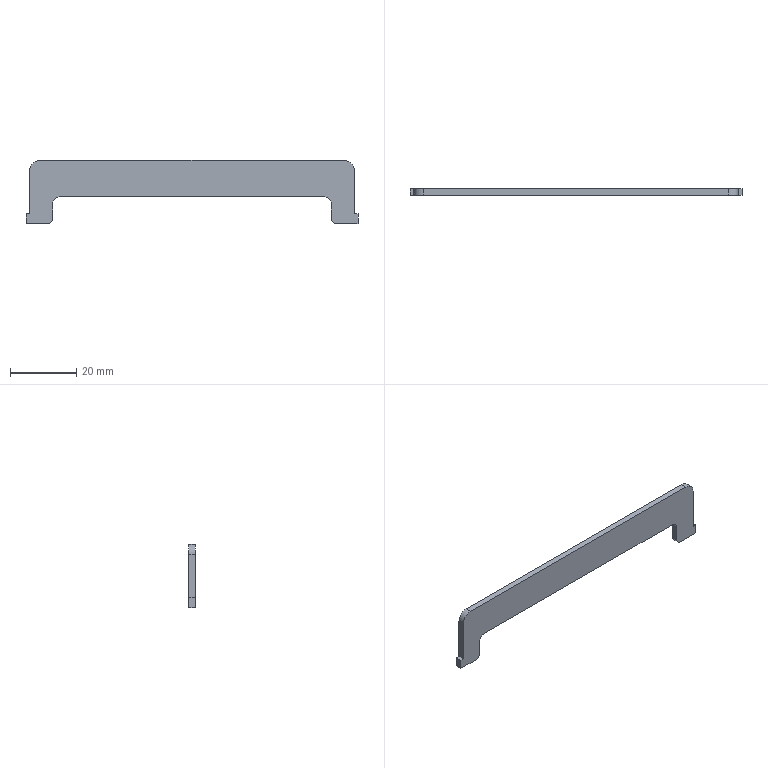Part | STEP file | 200 mesh_id2150 | 1 solid | 20 faces | box 100 x 1.9 x 19 mm | volume 2260 mm3 | plane 14 | cylinder 6 | commonest cylinder face diameters 3 x2 4 x2 6 x2
STEP:
#1=CARTESIAN_POINT('',(-16923.748,-4058.719,48.1));
#2=VERTEX_POINT('',#1);
#3=CARTESIAN_POINT('',(-17015.548,-4058.719,48.1));
#4=VERTEX_POINT('',#3);
#5=CARTESIAN_POINT('',(-16912.148,-4058.719,48.1));
#6=DIRECTION('',(-1.,0.,0.));
#7=VECTOR('',#6,1.);
#8=LINE('',#5,#7);
#9=EDGE_CURVE('',#2,#4,#8,.T.);
#10=ORIENTED_EDGE('',*,*,#9,.F.);
#11=CARTESIAN_POINT('',(-16923.748,-4056.819,48.1));
#12=VERTEX_POINT('',#11);
#13=CARTESIAN_POINT('',(-16923.748,-4058.744,48.1));
#14=DIRECTION('',(0.,1.,0.));
#15=VECTOR('',#14,1.);
#16=LINE('',#13,#15);
#17=EDGE_CURVE('',#2,#12,#16,.T.);
#18=ORIENTED_EDGE('',*,*,#17,.T.);
#19=CARTESIAN_POINT('',(-17015.548,-4056.819,48.1));
#20=VERTEX_POINT('',#19);
#21=CARTESIAN_POINT('',(-16912.148,-4056.819,48.1));
#22=DIRECTION('',(-1.,0.,0.));
#23=VECTOR('',#22,1.);
#24=LINE('',#21,#23);
#25=EDGE_CURVE('',#12,#20,#24,.T.);
#26=ORIENTED_EDGE('',*,*,#25,.T.);
#27=CARTESIAN_POINT('',(-17015.548,-4058.744,48.1));
#28=DIRECTION('',(0.,-1.,0.));
#29=VECTOR('',#28,1.);
#30=LINE('',#27,#29);
#31=EDGE_CURVE('',#20,#4,#30,.T.);
#32=ORIENTED_EDGE('',*,*,#31,.T.);
#33=EDGE_LOOP('',(#10,#18,#26,#32));
#34=FACE_OUTER_BOUND('',#33,.T.);
#35=CARTESIAN_POINT('',(-16912.148,-4058.744,48.1));
#36=DIRECTION('',(0.,0.,-1.));
#37=DIRECTION('',(1.,0.,0.));
#38=AXIS2_PLACEMENT_3D('',#35,#36,#37);
#39=PLANE('',#38);
#40=ADVANCED_FACE('',(#34),#39,.F.);
#41=CARTESIAN_POINT('',(-17018.548,-4058.719,45.1));
#42=VERTEX_POINT('',#41);
#43=CARTESIAN_POINT('',(-17018.548,-4058.719,32.1));
#44=VERTEX_POINT('',#43);
#45=CARTESIAN_POINT('',(-17018.548,-4058.719,46.6));
#46=DIRECTION('',(0.,0.,-1.));
#47=VECTOR('',#46,1.);
#48=LINE('',#45,#47);
#49=EDGE_CURVE('',#42,#44,#48,.T.);
#50=ORIENTED_EDGE('',*,*,#49,.F.);
#51=CARTESIAN_POINT('',(-17018.548,-4056.819,45.1));
#52=VERTEX_POINT('',#51);
#53=CARTESIAN_POINT('',(-17018.548,-4058.744,45.1));
#54=DIRECTION('',(0.,1.,0.));
#55=VECTOR('',#54,1.);
#56=LINE('',#53,#55);
#57=EDGE_CURVE('',#42,#52,#56,.T.);
#58=ORIENTED_EDGE('',*,*,#57,.T.);
#59=CARTESIAN_POINT('',(-17018.548,-4056.819,32.1));
#60=VERTEX_POINT('',#59);
#61=CARTESIAN_POINT('',(-17018.548,-4056.819,46.6));
#62=DIRECTION('',(0.,0.,-1.));
#63=VECTOR('',#62,1.);
#64=LINE('',#61,#63);
#65=EDGE_CURVE('',#52,#60,#64,.T.);
#66=ORIENTED_EDGE('',*,*,#65,.T.);
#67=CARTESIAN_POINT('',(-17018.548,-4058.744,32.1));
#68=DIRECTION('',(0.,1.,0.));
#69=VECTOR('',#68,1.);
#70=LINE('',#67,#69);
#71=EDGE_CURVE('',#44,#60,#70,.T.);
#72=ORIENTED_EDGE('',*,*,#71,.F.);
#73=EDGE_LOOP('',(#50,#58,#66,#72));
#74=FACE_OUTER_BOUND('',#73,.T.);
#75=CARTESIAN_POINT('',(-17018.548,-4058.744,46.6));
#76=DIRECTION('',(1.,0.,0.));
#77=DIRECTION('',(0.,1.,0.));
#78=AXIS2_PLACEMENT_3D('',#75,#76,#77);
#79=PLANE('',#78);
#80=ADVANCED_FACE('',(#74),#79,.F.);
#81=CARTESIAN_POINT('',(-17019.648,-4056.819,32.1));
#82=VERTEX_POINT('',#81);
#83=CARTESIAN_POINT('',(-17018.648,-4056.819,32.1));
#84=DIRECTION('',(-1.,0.,0.));
#85=VECTOR('',#84,1.);
#86=LINE('',#83,#85);
#87=EDGE_CURVE('',#60,#82,#86,.T.);
#88=ORIENTED_EDGE('',*,*,#87,.T.);
#89=CARTESIAN_POINT('',(-17019.648,-4058.719,32.1));
#90=VERTEX_POINT('',#89);
#91=CARTESIAN_POINT('',(-17019.648,-4058.744,32.1));
#92=DIRECTION('',(0.,1.,0.));
#93=VECTOR('',#92,1.);
#94=LINE('',#91,#93);
#95=EDGE_CURVE('',#90,#82,#94,.T.);
#96=ORIENTED_EDGE('',*,*,#95,.F.);
#97=CARTESIAN_POINT('',(-17018.648,-4058.719,32.1));
#98=DIRECTION('',(-1.,0.,0.));
#99=VECTOR('',#98,1.);
#100=LINE('',#97,#99);
#101=EDGE_CURVE('',#44,#90,#100,.T.);
#102=ORIENTED_EDGE('',*,*,#101,.F.);
#103=ORIENTED_EDGE('',*,*,#71,.T.);
#104=EDGE_LOOP('',(#88,#96,#102,#103));
#105=FACE_OUTER_BOUND('',#104,.T.);
#106=CARTESIAN_POINT('',(-17018.648,-4058.744,32.1));
#107=DIRECTION('',(0.,0.,-1.));
#108=DIRECTION('',(0.,1.,0.));
#109=AXIS2_PLACEMENT_3D('',#106,#107,#108);
#110=PLANE('',#109);
#111=ADVANCED_FACE('',(#105),#110,.F.);
#112=CARTESIAN_POINT('',(-17019.648,-4056.819,29.1));
#113=VERTEX_POINT('',#112);
#114=CARTESIAN_POINT('',(-17019.648,-4056.819,32.1));
#115=DIRECTION('',(0.,0.,-1.));
#116=VECTOR('',#115,1.);
#117=LINE('',#114,#116);
#118=EDGE_CURVE('',#82,#113,#117,.T.);
#119=ORIENTED_EDGE('',*,*,#118,.T.);
#120=CARTESIAN_POINT('',(-17019.648,-4058.719,29.1));
#121=VERTEX_POINT('',#120);
#122=CARTESIAN_POINT('',(-17019.648,-4058.744,29.1));
#123=DIRECTION('',(0.,1.,0.));
#124=VECTOR('',#123,1.);
#125=LINE('',#122,#124);
#126=EDGE_CURVE('',#121,#113,#125,.T.);
#127=ORIENTED_EDGE('',*,*,#126,.F.);
#128=CARTESIAN_POINT('',(-17019.648,-4058.719,32.1));
#129=DIRECTION('',(0.,0.,-1.));
#130=VECTOR('',#129,1.);
#131=LINE('',#128,#130);
#132=EDGE_CURVE('',#90,#121,#131,.T.);
#133=ORIENTED_EDGE('',*,*,#132,.F.);
#134=ORIENTED_EDGE('',*,*,#95,.T.);
#135=EDGE_LOOP('',(#119,#127,#133,#134));
#136=FACE_OUTER_BOUND('',#135,.T.);
#137=CARTESIAN_POINT('',(-17019.648,-4058.744,32.1));
#138=DIRECTION('',(1.,0.,0.));
#139=DIRECTION('',(0.,1.,0.));
#140=AXIS2_PLACEMENT_3D('',#137,#138,#139);
#141=PLANE('',#140);
#142=ADVANCED_FACE('',(#136),#141,.F.);
#143=CARTESIAN_POINT('',(-17013.148,-4056.819,29.1));
#144=VERTEX_POINT('',#143);
#145=CARTESIAN_POINT('',(-17019.648,-4056.819,29.1));
#146=DIRECTION('',(1.,0.,0.));
#147=VECTOR('',#146,1.);
#148=LINE('',#145,#147);
#149=EDGE_CURVE('',#113,#144,#148,.T.);
#150=ORIENTED_EDGE('',*,*,#149,.T.);
#151=CARTESIAN_POINT('',(-17013.148,-4058.719,29.1));
#152=VERTEX_POINT('',#151);
#153=CARTESIAN_POINT('',(-17013.148,-4058.744,29.1));
#154=DIRECTION('',(0.,-1.,0.));
#155=VECTOR('',#154,1.);
#156=LINE('',#153,#155);
#157=EDGE_CURVE('',#144,#152,#156,.T.);
#158=ORIENTED_EDGE('',*,*,#157,.T.);
#159=CARTESIAN_POINT('',(-17019.648,-4058.719,29.1));
#160=DIRECTION('',(1.,0.,0.));
#161=VECTOR('',#160,1.);
#162=LINE('',#159,#161);
#163=EDGE_CURVE('',#121,#152,#162,.T.);
#164=ORIENTED_EDGE('',*,*,#163,.F.);
#165=ORIENTED_EDGE('',*,*,#126,.T.);
#166=EDGE_LOOP('',(#150,#158,#164,#165));
#167=FACE_OUTER_BOUND('',#166,.T.);
#168=CARTESIAN_POINT('',(-17019.648,-4058.744,29.1));
#169=DIRECTION('',(0.,0.,1.));
#170=DIRECTION('',(0.,-1.,0.));
#171=AXIS2_PLACEMENT_3D('',#168,#169,#170);
#172=PLANE('',#171);
#173=ADVANCED_FACE('',(#167),#172,.F.);
#174=CARTESIAN_POINT('',(-17011.648,-4058.719,30.6));
#175=VERTEX_POINT('',#174);
#176=CARTESIAN_POINT('',(-17011.648,-4058.719,35.1));
#177=VERTEX_POINT('',#176);
#178=CARTESIAN_POINT('',(-17011.648,-4058.719,29.1));
#179=DIRECTION('',(0.,0.,1.));
#180=VECTOR('',#179,1.);
#181=LINE('',#178,#180);
#182=EDGE_CURVE('',#175,#177,#181,.T.);
#183=ORIENTED_EDGE('',*,*,#182,.F.);
#184=CARTESIAN_POINT('',(-17011.648,-4056.819,30.6));
#185=VERTEX_POINT('',#184);
#186=CARTESIAN_POINT('',(-17011.648,-4058.744,30.6));
#187=DIRECTION('',(0.,1.,0.));
#188=VECTOR('',#187,1.);
#189=LINE('',#186,#188);
#190=EDGE_CURVE('',#175,#185,#189,.T.);
#191=ORIENTED_EDGE('',*,*,#190,.T.);
#192=CARTESIAN_POINT('',(-17011.648,-4056.819,35.1));
#193=VERTEX_POINT('',#192);
#194=CARTESIAN_POINT('',(-17011.648,-4056.819,29.1));
#195=DIRECTION('',(0.,0.,1.));
#196=VECTOR('',#195,1.);
#197=LINE('',#194,#196);
#198=EDGE_CURVE('',#185,#193,#197,.T.);
#199=ORIENTED_EDGE('',*,*,#198,.T.);
#200=CARTESIAN_POINT('',(-17011.648,-4058.744,35.1));
#201=DIRECTION('',(0.,-1.,0.));
#202=VECTOR('',#201,1.);
#203=LINE('',#200,#202);
#204=EDGE_CURVE('',#193,#177,#203,.T.);
#205=ORIENTED_EDGE('',*,*,#204,.T.);
#206=EDGE_LOOP('',(#183,#191,#199,#205));
#207=FACE_OUTER_BOUND('',#206,.T.);
#208=CARTESIAN_POINT('',(-17011.648,-4058.744,29.1));
#209=DIRECTION('',(-1.,0.,0.));
#210=DIRECTION('',(0.,-1.,0.));
#211=AXIS2_PLACEMENT_3D('',#208,#209,#210);
#212=PLANE('',#211);
#213=ADVANCED_FACE('',(#207),#212,.F.);
#214=CARTESIAN_POINT('',(-17009.648,-4058.719,37.1));
#215=VERTEX_POINT('',#214);
#216=CARTESIAN_POINT('',(-16929.648,-4058.719,37.1));
#217=VERTEX_POINT('',#216);
#218=CARTESIAN_POINT('',(-17015.648,-4058.719,37.1));
#219=DIRECTION('',(1.,0.,0.));
#220=VECTOR('',#219,1.);
#221=LINE('',#218,#220);
#222=EDGE_CURVE('',#215,#217,#221,.T.);
#223=ORIENTED_EDGE('',*,*,#222,.F.);
#224=CARTESIAN_POINT('',(-17009.648,-4056.819,37.1));
#225=VERTEX_POINT('',#224);
#226=CARTESIAN_POINT('',(-17009.648,-4058.744,37.1));
#227=DIRECTION('',(0.,1.,0.));
#228=VECTOR('',#227,1.);
#229=LINE('',#226,#228);
#230=EDGE_CURVE('',#215,#225,#229,.T.);
#231=ORIENTED_EDGE('',*,*,#230,.T.);
#232=CARTESIAN_POINT('',(-16929.648,-4056.819,37.1));
#233=VERTEX_POINT('',#232);
#234=CARTESIAN_POINT('',(-17015.648,-4056.819,37.1));
#235=DIRECTION('',(1.,0.,0.));
#236=VECTOR('',#235,1.);
#237=LINE('',#234,#236);
#238=EDGE_CURVE('',#225,#233,#237,.T.);
#239=ORIENTED_EDGE('',*,*,#238,.T.);
#240=CARTESIAN_POINT('',(-16929.648,-4058.744,37.1));
#241=DIRECTION('',(0.,-1.,0.));
#242=VECTOR('',#241,1.);
#243=LINE('',#240,#242);
#244=EDGE_CURVE('',#233,#217,#243,.T.);
#245=ORIENTED_EDGE('',*,*,#244,.T.);
#246=EDGE_LOOP('',(#223,#231,#239,#245));
#247=FACE_OUTER_BOUND('',#246,.T.);
#248=CARTESIAN_POINT('',(-17015.648,-4058.744,37.1));
#249=DIRECTION('',(0.,0.,1.));
#250=DIRECTION('',(0.,-1.,0.));
#251=AXIS2_PLACEMENT_3D('',#248,#249,#250);
#252=PLANE('',#251);
#253=ADVANCED_FACE('',(#247),#252,.F.);
#254=CARTESIAN_POINT('',(-16927.648,-4056.819,35.1));
#255=VERTEX_POINT('',#254);
#256=CARTESIAN_POINT('',(-16927.648,-4056.819,30.6));
#257=VERTEX_POINT('',#256);
#258=CARTESIAN_POINT('',(-16927.648,-4056.819,37.1));
#259=DIRECTION('',(0.,0.,-1.));
#260=VECTOR('',#259,1.);
#261=LINE('',#258,#260);
#262=EDGE_CURVE('',#255,#257,#261,.T.);
#263=ORIENTED_EDGE('',*,*,#262,.T.);
#264=CARTESIAN_POINT('',(-16927.648,-4058.719,30.6));
#265=VERTEX_POINT('',#264);
#266=CARTESIAN_POINT('',(-16927.648,-4058.744,30.6));
#267=DIRECTION('',(0.,-1.,0.));
#268=VECTOR('',#267,1.);
#269=LINE('',#266,#268);
#270=EDGE_CURVE('',#257,#265,#269,.T.);
#271=ORIENTED_EDGE('',*,*,#270,.T.);
#272=CARTESIAN_POINT('',(-16927.648,-4058.719,35.1));
#273=VERTEX_POINT('',#272);
#274=CARTESIAN_POINT('',(-16927.648,-4058.719,37.1));
#275=DIRECTION('',(0.,0.,-1.));
#276=VECTOR('',#275,1.);
#277=LINE('',#274,#276);
#278=EDGE_CURVE('',#273,#265,#277,.T.);
#279=ORIENTED_EDGE('',*,*,#278,.F.);
#280=CARTESIAN_POINT('',(-16927.648,-4058.744,35.1));
#281=DIRECTION('',(0.,1.,0.));
#282=VECTOR('',#281,1.);
#283=LINE('',#280,#282);
#284=EDGE_CURVE('',#273,#255,#283,.T.);
#285=ORIENTED_EDGE('',*,*,#284,.T.);
#286=EDGE_LOOP('',(#263,#271,#279,#285));
#287=FACE_OUTER_BOUND('',#286,.T.);
#288=CARTESIAN_POINT('',(-16927.648,-4058.744,37.1));
#289=DIRECTION('',(1.,0.,0.));
#290=DIRECTION('',(0.,1.,0.));
#291=AXIS2_PLACEMENT_3D('',#288,#289,#290);
#292=PLANE('',#291);
#293=ADVANCED_FACE('',(#287),#292,.F.);
#294=CARTESIAN_POINT('',(-16926.148,-4058.719,29.1));
#295=VERTEX_POINT('',#294);
#296=CARTESIAN_POINT('',(-16919.648,-4058.719,29.1));
#297=VERTEX_POINT('',#296);
#298=CARTESIAN_POINT('',(-16930.648,-4058.719,29.1));
#299=DIRECTION('',(1.,0.,0.));
#300=VECTOR('',#299,1.);
#301=LINE('',#298,#300);
#302=EDGE_CURVE('',#295,#297,#301,.T.);
#303=ORIENTED_EDGE('',*,*,#302,.F.);
#304=CARTESIAN_POINT('',(-16926.148,-4056.819,29.1));
#305=VERTEX_POINT('',#304);
#306=CARTESIAN_POINT('',(-16926.148,-4058.744,29.1));
#307=DIRECTION('',(0.,1.,0.));
#308=VECTOR('',#307,1.);
#309=LINE('',#306,#308);
#310=EDGE_CURVE('',#295,#305,#309,.T.);
#311=ORIENTED_EDGE('',*,*,#310,.T.);
#312=CARTESIAN_POINT('',(-16919.648,-4056.819,29.1));
#313=VERTEX_POINT('',#312);
#314=CARTESIAN_POINT('',(-16930.648,-4056.819,29.1));
#315=DIRECTION('',(1.,0.,0.));
#316=VECTOR('',#315,1.);
#317=LINE('',#314,#316);
#318=EDGE_CURVE('',#305,#313,#317,.T.);
#319=ORIENTED_EDGE('',*,*,#318,.T.);
#320=CARTESIAN_POINT('',(-16919.648,-4058.744,29.1));
#321=DIRECTION('',(0.,1.,0.));
#322=VECTOR('',#321,1.);
#323=LINE('',#320,#322);
#324=EDGE_CURVE('',#297,#313,#323,.T.);
#325=ORIENTED_EDGE('',*,*,#324,.F.);
#326=EDGE_LOOP('',(#303,#311,#319,#325));
#327=FACE_OUTER_BOUND('',#326,.T.);
#328=CARTESIAN_POINT('',(-16930.648,-4058.744,29.1));
#329=DIRECTION('',(0.,0.,1.));
#330=DIRECTION('',(0.,-1.,0.));
#331=AXIS2_PLACEMENT_3D('',#328,#329,#330);
#332=PLANE('',#331);
#333=ADVANCED_FACE('',(#327),#332,.F.);
#334=CARTESIAN_POINT('',(-16919.648,-4056.819,32.1));
#335=VERTEX_POINT('',#334);
#336=CARTESIAN_POINT('',(-16919.648,-4056.819,29.1));
#337=DIRECTION('',(0.,0.,1.));
#338=VECTOR('',#337,1.);
#339=LINE('',#336,#338);
#340=EDGE_CURVE('',#313,#335,#339,.T.);
#341=ORIENTED_EDGE('',*,*,#340,.T.);
#342=CARTESIAN_POINT('',(-16919.648,-4058.719,32.1));
#343=VERTEX_POINT('',#342);
#344=CARTESIAN_POINT('',(-16919.648,-4058.744,32.1));
#345=DIRECTION('',(0.,1.,0.));
#346=VECTOR('',#345,1.);
#347=LINE('',#344,#346);
#348=EDGE_CURVE('',#343,#335,#347,.T.);
#349=ORIENTED_EDGE('',*,*,#348,.F.);
#350=CARTESIAN_POINT('',(-16919.648,-4058.719,29.1));
#351=DIRECTION('',(0.,0.,1.));
#352=VECTOR('',#351,1.);
#353=LINE('',#350,#352);
#354=EDGE_CURVE('',#297,#343,#353,.T.);
#355=ORIENTED_EDGE('',*,*,#354,.F.);
#356=ORIENTED_EDGE('',*,*,#324,.T.);
#357=EDGE_LOOP('',(#341,#349,#355,#356));
#358=FACE_OUTER_BOUND('',#357,.T.);
#359=CARTESIAN_POINT('',(-16919.648,-4058.744,29.1));
#360=DIRECTION('',(-1.,0.,0.));
#361=DIRECTION('',(0.,-1.,0.));
#362=AXIS2_PLACEMENT_3D('',#359,#360,#361);
#363=PLANE('',#362);
#364=ADVANCED_FACE('',(#358),#363,.F.);
#365=CARTESIAN_POINT('',(-16920.748,-4056.819,32.1));
#366=VERTEX_POINT('',#365);
#367=CARTESIAN_POINT('',(-16919.648,-4056.819,32.1));
#368=DIRECTION('',(-1.,0.,0.));
#369=VECTOR('',#368,1.);
#370=LINE('',#367,#369);
#371=EDGE_CURVE('',#335,#366,#370,.T.);
#372=ORIENTED_EDGE('',*,*,#371,.T.);
#373=CARTESIAN_POINT('',(-16920.748,-4058.719,32.1));
#374=VERTEX_POINT('',#373);
#375=CARTESIAN_POINT('',(-16920.748,-4058.744,32.1));
#376=DIRECTION('',(0.,1.,0.));
#377=VECTOR('',#376,1.);
#378=LINE('',#375,#377);
#379=EDGE_CURVE('',#374,#366,#378,.T.);
#380=ORIENTED_EDGE('',*,*,#379,.F.);
#381=CARTESIAN_POINT('',(-16919.648,-4058.719,32.1));
#382=DIRECTION('',(-1.,0.,0.));
#383=VECTOR('',#382,1.);
#384=LINE('',#381,#383);
#385=EDGE_CURVE('',#343,#374,#384,.T.);
#386=ORIENTED_EDGE('',*,*,#385,.F.);
#387=ORIENTED_EDGE('',*,*,#348,.T.);
#388=EDGE_LOOP('',(#372,#380,#386,#387));
#389=FACE_OUTER_BOUND('',#388,.T.);
#390=CARTESIAN_POINT('',(-16919.648,-4058.744,32.1));
#391=DIRECTION('',(0.,0.,-1.));
#392=DIRECTION('',(0.,1.,0.));
#393=AXIS2_PLACEMENT_3D('',#390,#391,#392);
#394=PLANE('',#393);
#395=ADVANCED_FACE('',(#389),#394,.F.);
#396=CARTESIAN_POINT('',(-16920.748,-4056.819,45.1));
#397=VERTEX_POINT('',#396);
#398=CARTESIAN_POINT('',(-16920.748,-4056.819,32.1));
#399=DIRECTION('',(0.,0.,1.));
#400=VECTOR('',#399,1.);
#401=LINE('',#398,#400);
#402=EDGE_CURVE('',#366,#397,#401,.T.);
#403=ORIENTED_EDGE('',*,*,#402,.T.);
#404=CARTESIAN_POINT('',(-16920.748,-4058.719,45.1));
#405=VERTEX_POINT('',#404);
#406=CARTESIAN_POINT('',(-16920.748,-4058.744,45.1));
#407=DIRECTION('',(0.,-1.,0.));
#408=VECTOR('',#407,1.);
#409=LINE('',#406,#408);
#410=EDGE_CURVE('',#397,#405,#409,.T.);
#411=ORIENTED_EDGE('',*,*,#410,.T.);
#412=CARTESIAN_POINT('',(-16920.748,-4058.719,32.1));
#413=DIRECTION('',(0.,0.,1.));
#414=VECTOR('',#413,1.);
#415=LINE('',#412,#414);
#416=EDGE_CURVE('',#374,#405,#415,.T.);
#417=ORIENTED_EDGE('',*,*,#416,.F.);
#418=ORIENTED_EDGE('',*,*,#379,.T.);
#419=EDGE_LOOP('',(#403,#411,#417,#418));
#420=FACE_OUTER_BOUND('',#419,.T.);
#421=CARTESIAN_POINT('',(-16920.748,-4058.744,32.1));
#422=DIRECTION('',(-1.,0.,0.));
#423=DIRECTION('',(0.,-1.,0.));
#424=AXIS2_PLACEMENT_3D('',#421,#422,#423);
#425=PLANE('',#424);
#426=ADVANCED_FACE('',(#420),#425,.F.);
#427=ORIENTED_EDGE('',*,*,#278,.T.);
#428=CARTESIAN_POINT('',(-16926.148,-4058.719,30.6));
#429=DIRECTION('',(0.,-1.,0.));
#430=DIRECTION('',(0.,0.,-1.));
#431=AXIS2_PLACEMENT_3D('',#428,#429,#430);
#432=CIRCLE('',#431,1.5);
#433=EDGE_CURVE('',#265,#295,#432,.T.);
#434=ORIENTED_EDGE('',*,*,#433,.T.);
#435=ORIENTED_EDGE('',*,*,#302,.T.);
#436=ORIENTED_EDGE('',*,*,#354,.T.);
#437=ORIENTED_EDGE('',*,*,#385,.T.);
#438=ORIENTED_EDGE('',*,*,#416,.T.);
#439=CARTESIAN_POINT('',(-16923.748,-4058.719,45.1));
#440=DIRECTION('',(0.,-1.,0.));
#441=DIRECTION('',(0.,0.,-1.));
#442=AXIS2_PLACEMENT_3D('',#439,#440,#441);
#443=CIRCLE('',#442,3.);
#444=EDGE_CURVE('',#405,#2,#443,.T.);
#445=ORIENTED_EDGE('',*,*,#444,.T.);
#446=ORIENTED_EDGE('',*,*,#9,.T.);
#447=CARTESIAN_POINT('',(-17015.548,-4058.719,45.1));
#448=DIRECTION('',(0.,-1.,0.));
#449=DIRECTION('',(0.,0.,-1.));
#450=AXIS2_PLACEMENT_3D('',#447,#448,#449);
#451=CIRCLE('',#450,3.);
#452=EDGE_CURVE('',#4,#42,#451,.T.);
#453=ORIENTED_EDGE('',*,*,#452,.T.);
#454=ORIENTED_EDGE('',*,*,#49,.T.);
#455=ORIENTED_EDGE('',*,*,#101,.T.);
#456=ORIENTED_EDGE('',*,*,#132,.T.);
#457=ORIENTED_EDGE('',*,*,#163,.T.);
#458=CARTESIAN_POINT('',(-17013.148,-4058.719,30.6));
#459=DIRECTION('',(0.,-1.,0.));
#460=DIRECTION('',(0.,0.,-1.));
#461=AXIS2_PLACEMENT_3D('',#458,#459,#460);
#462=CIRCLE('',#461,1.5);
#463=EDGE_CURVE('',#152,#175,#462,.T.);
#464=ORIENTED_EDGE('',*,*,#463,.T.);
#465=ORIENTED_EDGE('',*,*,#182,.T.);
#466=CARTESIAN_POINT('',(-17009.648,-4058.719,35.1));
#467=DIRECTION('',(0.,1.,0.));
#468=DIRECTION('',(0.,0.,-1.));
#469=AXIS2_PLACEMENT_3D('',#466,#467,#468);
#470=CIRCLE('',#469,2.);
#471=EDGE_CURVE('',#177,#215,#470,.T.);
#472=ORIENTED_EDGE('',*,*,#471,.T.);
#473=ORIENTED_EDGE('',*,*,#222,.T.);
#474=CARTESIAN_POINT('',(-16929.648,-4058.719,35.1));
#475=DIRECTION('',(0.,1.,0.));
#476=DIRECTION('',(0.,0.,-1.));
#477=AXIS2_PLACEMENT_3D('',#474,#475,#476);
#478=CIRCLE('',#477,2.);
#479=EDGE_CURVE('',#217,#273,#478,.T.);
#480=ORIENTED_EDGE('',*,*,#479,.T.);
#481=EDGE_LOOP('',(#427,#434,#435,#436,#437,#438,#445,#446,#453,#454,#455,#456,#457,#464,#465,#472,#473,#480));
#482=FACE_OUTER_BOUND('',#481,.T.);
#483=CARTESIAN_POINT('',(-17024.148,-4058.719,46.6));
#484=DIRECTION('',(0.,-1.,0.));
#485=DIRECTION('',(1.,0.,0.));
#486=AXIS2_PLACEMENT_3D('',#483,#484,#485);
#487=PLANE('',#486);
#488=ADVANCED_FACE('',(#482),#487,.T.);
#489=ORIENTED_EDGE('',*,*,#318,.F.);
#490=CARTESIAN_POINT('',(-16926.148,-4056.819,30.6));
#491=DIRECTION('',(0.,1.,0.));
#492=DIRECTION('',(0.,0.,-1.));
#493=AXIS2_PLACEMENT_3D('',#490,#491,#492);
#494=CIRCLE('',#493,1.5);
#495=EDGE_CURVE('',#305,#257,#494,.T.);
#496=ORIENTED_EDGE('',*,*,#495,.T.);
#497=ORIENTED_EDGE('',*,*,#262,.F.);
#498=CARTESIAN_POINT('',(-16929.648,-4056.819,35.1));
#499=DIRECTION('',(0.,-1.,0.));
#500=DIRECTION('',(0.,0.,-1.));
#501=AXIS2_PLACEMENT_3D('',#498,#499,#500);
#502=CIRCLE('',#501,2.);
#503=EDGE_CURVE('',#255,#233,#502,.T.);
#504=ORIENTED_EDGE('',*,*,#503,.T.);
#505=ORIENTED_EDGE('',*,*,#238,.F.);
#506=CARTESIAN_POINT('',(-17009.648,-4056.819,35.1));
#507=DIRECTION('',(0.,-1.,0.));
#508=DIRECTION('',(0.,0.,-1.));
#509=AXIS2_PLACEMENT_3D('',#506,#507,#508);
#510=CIRCLE('',#509,2.);
#511=EDGE_CURVE('',#225,#193,#510,.T.);
#512=ORIENTED_EDGE('',*,*,#511,.T.);
#513=ORIENTED_EDGE('',*,*,#198,.F.);
#514=CARTESIAN_POINT('',(-17013.148,-4056.819,30.6));
#515=DIRECTION('',(0.,1.,0.));
#516=DIRECTION('',(0.,0.,-1.));
#517=AXIS2_PLACEMENT_3D('',#514,#515,#516);
#518=CIRCLE('',#517,1.5);
#519=EDGE_CURVE('',#185,#144,#518,.T.);
#520=ORIENTED_EDGE('',*,*,#519,.T.);
#521=ORIENTED_EDGE('',*,*,#149,.F.);
#522=ORIENTED_EDGE('',*,*,#118,.F.);
#523=ORIENTED_EDGE('',*,*,#87,.F.);
#524=ORIENTED_EDGE('',*,*,#65,.F.);
#525=CARTESIAN_POINT('',(-17015.548,-4056.819,45.1));
#526=DIRECTION('',(0.,1.,0.));
#527=DIRECTION('',(0.,0.,-1.));
#528=AXIS2_PLACEMENT_3D('',#525,#526,#527);
#529=CIRCLE('',#528,3.);
#530=EDGE_CURVE('',#52,#20,#529,.T.);
#531=ORIENTED_EDGE('',*,*,#530,.T.);
#532=ORIENTED_EDGE('',*,*,#25,.F.);
#533=CARTESIAN_POINT('',(-16923.748,-4056.819,45.1));
#534=DIRECTION('',(0.,1.,0.));
#535=DIRECTION('',(0.,0.,-1.));
#536=AXIS2_PLACEMENT_3D('',#533,#534,#535);
#537=CIRCLE('',#536,3.);
#538=EDGE_CURVE('',#12,#397,#537,.T.);
#539=ORIENTED_EDGE('',*,*,#538,.T.);
#540=ORIENTED_EDGE('',*,*,#402,.F.);
#541=ORIENTED_EDGE('',*,*,#371,.F.);
#542=ORIENTED_EDGE('',*,*,#340,.F.);
#543=EDGE_LOOP('',(#489,#496,#497,#504,#505,#512,#513,#520,#521,#522,#523,#524,#531,#532,#539,#540,#541,#542));
#544=FACE_OUTER_BOUND('',#543,.T.);
#545=CARTESIAN_POINT('',(-17024.148,-4056.819,46.6));
#546=DIRECTION('',(0.,-1.,0.));
#547=DIRECTION('',(1.,0.,0.));
#548=AXIS2_PLACEMENT_3D('',#545,#546,#547);
#549=PLANE('',#548);
#550=ADVANCED_FACE('',(#544),#549,.F.);
#551=ORIENTED_EDGE('',*,*,#479,.F.);
#552=ORIENTED_EDGE('',*,*,#244,.F.);
#553=ORIENTED_EDGE('',*,*,#503,.F.);
#554=ORIENTED_EDGE('',*,*,#284,.F.);
#555=EDGE_LOOP('',(#551,#552,#553,#554));
#556=FACE_OUTER_BOUND('',#555,.T.);
#557=CARTESIAN_POINT('',(-16929.648,-4058.744,35.1));
#558=DIRECTION('',(0.,1.,0.));
#559=DIRECTION('',(0.,0.,1.));
#560=AXIS2_PLACEMENT_3D('',#557,#558,#559);
#561=CYLINDRICAL_SURFACE('',#560,2.);
#562=ADVANCED_FACE('',(#556),#561,.F.);
#563=ORIENTED_EDGE('',*,*,#471,.F.);
#564=ORIENTED_EDGE('',*,*,#204,.F.);
#565=ORIENTED_EDGE('',*,*,#511,.F.);
#566=ORIENTED_EDGE('',*,*,#230,.F.);
#567=EDGE_LOOP('',(#563,#564,#565,#566));
#568=FACE_OUTER_BOUND('',#567,.T.);
#569=CARTESIAN_POINT('',(-17009.648,-4058.744,35.1));
#570=DIRECTION('',(0.,1.,0.));
#571=DIRECTION('',(0.,0.,1.));
#572=AXIS2_PLACEMENT_3D('',#569,#570,#571);
#573=CYLINDRICAL_SURFACE('',#572,2.);
#574=ADVANCED_FACE('',(#568),#573,.F.);
#575=ORIENTED_EDGE('',*,*,#444,.F.);
#576=ORIENTED_EDGE('',*,*,#410,.F.);
#577=ORIENTED_EDGE('',*,*,#538,.F.);
#578=ORIENTED_EDGE('',*,*,#17,.F.);
#579=EDGE_LOOP('',(#575,#576,#577,#578));
#580=FACE_OUTER_BOUND('',#579,.T.);
#581=CARTESIAN_POINT('',(-16923.748,-4058.744,45.1));
#582=DIRECTION('',(0.,1.,0.));
#583=DIRECTION('',(0.,0.,1.));
#584=AXIS2_PLACEMENT_3D('',#581,#582,#583);
#585=CYLINDRICAL_SURFACE('',#584,3.);
#586=ADVANCED_FACE('',(#580),#585,.T.);
#587=ORIENTED_EDGE('',*,*,#452,.F.);
#588=ORIENTED_EDGE('',*,*,#31,.F.);
#589=ORIENTED_EDGE('',*,*,#530,.F.);
#590=ORIENTED_EDGE('',*,*,#57,.F.);
#591=EDGE_LOOP('',(#587,#588,#589,#590));
#592=FACE_OUTER_BOUND('',#591,.T.);
#593=CARTESIAN_POINT('',(-17015.548,-4058.744,45.1));
#594=DIRECTION('',(0.,1.,0.));
#595=DIRECTION('',(0.,0.,1.));
#596=AXIS2_PLACEMENT_3D('',#593,#594,#595);
#597=CYLINDRICAL_SURFACE('',#596,3.);
#598=ADVANCED_FACE('',(#592),#597,.T.);
#599=ORIENTED_EDGE('',*,*,#433,.F.);
#600=ORIENTED_EDGE('',*,*,#270,.F.);
#601=ORIENTED_EDGE('',*,*,#495,.F.);
#602=ORIENTED_EDGE('',*,*,#310,.F.);
#603=EDGE_LOOP('',(#599,#600,#601,#602));
#604=FACE_OUTER_BOUND('',#603,.T.);
#605=CARTESIAN_POINT('',(-16926.148,-4058.744,30.6));
#606=DIRECTION('',(0.,1.,0.));
#607=DIRECTION('',(0.,0.,1.));
#608=AXIS2_PLACEMENT_3D('',#605,#606,#607);
#609=CYLINDRICAL_SURFACE('',#608,1.5);
#610=ADVANCED_FACE('',(#604),#609,.T.);
#611=ORIENTED_EDGE('',*,*,#463,.F.);
#612=ORIENTED_EDGE('',*,*,#157,.F.);
#613=ORIENTED_EDGE('',*,*,#519,.F.);
#614=ORIENTED_EDGE('',*,*,#190,.F.);
#615=EDGE_LOOP('',(#611,#612,#613,#614));
#616=FACE_OUTER_BOUND('',#615,.T.);
#617=CARTESIAN_POINT('',(-17013.148,-4058.744,30.6));
#618=DIRECTION('',(0.,1.,0.));
#619=DIRECTION('',(0.,0.,1.));
#620=AXIS2_PLACEMENT_3D('',#617,#618,#619);
#621=CYLINDRICAL_SURFACE('',#620,1.5);
#622=ADVANCED_FACE('',(#616),#621,.T.);
#623=CLOSED_SHELL('',(#40,#80,#111,#142,#173,#213,#253,#293,#333,#364,#395,#426,#488,#550,#562,#574,#586,#598,#610,#622));
#624=MANIFOLD_SOLID_BREP('',#623);
#625=(LENGTH_UNIT()NAMED_UNIT(*)SI_UNIT(.MILLI.,.METRE.));
#626=UNCERTAINTY_MEASURE_WITH_UNIT(LENGTH_MEASURE(0.00002),#625,'','');
#627=(NAMED_UNIT(*)PLANE_ANGLE_UNIT()SI_UNIT($,.RADIAN.));
#628=PLANE_ANGLE_MEASURE_WITH_UNIT(PLANE_ANGLE_MEASURE(0.01745),#627);
#629=DIMENSIONAL_EXPONENTS(0.,0.,0.,0.,0.,0.,0.);
#630=(CONVERSION_BASED_UNIT('DEGREE',#628)NAMED_UNIT(#629)PLANE_ANGLE_UNIT());
#631=(NAMED_UNIT(*)SI_UNIT($,.STERADIAN.)SOLID_ANGLE_UNIT());
#632=(GEOMETRIC_REPRESENTATION_CONTEXT(3)GLOBAL_UNCERTAINTY_ASSIGNED_CONTEXT((#626))GLOBAL_UNIT_ASSIGNED_CONTEXT((#625,#630,#631))REPRESENTATION_CONTEXT('',''));
#633=ADVANCED_BREP_SHAPE_REPRESENTATION('',(#624),#632);